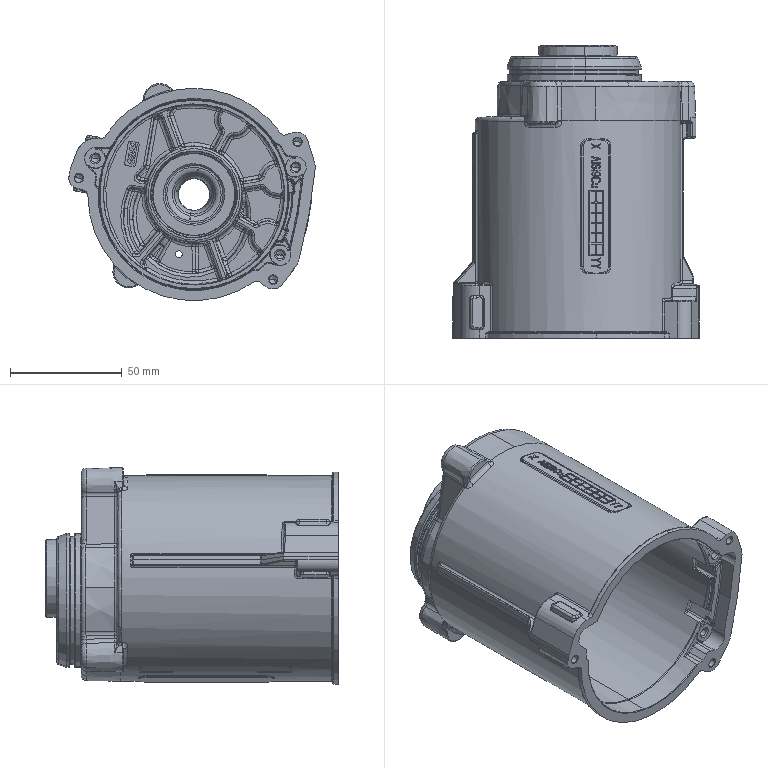Part | SolidWorks | features BaseBody 1 | 1 solid | 1600 faces | box 110.214 x 131 x 97.13 mm | volume 198684 mm3 | plane 518 | spline 385 | cylinder 309 | torus 184 | cone 141 | sphere 63 | commonest cylinder face diameters 1 x75 0.5 x56 2 x51 3 x36 3.66 x12 0.6 x11